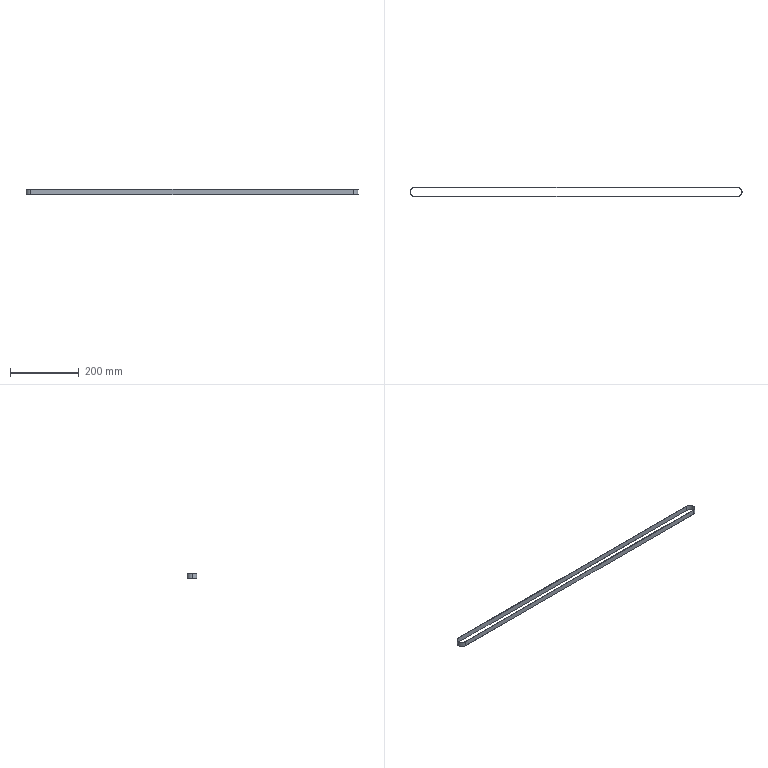Part | SolidWorks | features Extrusion 1 | 1 solid | 12 faces | box 965.34 x 28.34 x 15 mm | volume 34680 mm3 | cylinder 6 | plane 6 | commonest cylinder face diameters 25.98 x3 28.34 x3
STEP:
#1=CARTESIAN_POINT('',(0.,12.99,7.5));
#2=VERTEX_POINT('',#1);
#3=CARTESIAN_POINT('',(-12.99,0.,7.5));
#4=VERTEX_POINT('',#3);
#5=CARTESIAN_POINT('',(0.,0.,7.5));
#6=DIRECTION('',(0.,0.,1.));
#7=DIRECTION('',(1.,0.,0.));
#8=AXIS2_PLACEMENT_3D('',#5,#6,#7);
#9=CIRCLE('',#8,12.99);
#10=EDGE_CURVE('',#2,#4,#9,.T.);
#11=ORIENTED_EDGE('',*,*,#10,.T.);
#12=CARTESIAN_POINT('',(-12.99,0.,-7.5));
#13=VERTEX_POINT('',#12);
#14=CARTESIAN_POINT('',(-12.99,0.,7.5));
#15=DIRECTION('',(0.,0.,-1.));
#16=VECTOR('',#15,1000.);
#17=LINE('',#14,#16);
#18=EDGE_CURVE('',#4,#13,#17,.T.);
#19=ORIENTED_EDGE('',*,*,#18,.T.);
#20=CARTESIAN_POINT('',(0.,12.99,-7.5));
#21=VERTEX_POINT('',#20);
#22=CARTESIAN_POINT('',(0.,0.,-7.5));
#23=DIRECTION('',(0.,0.,1.));
#24=DIRECTION('',(1.,0.,0.));
#25=AXIS2_PLACEMENT_3D('',#22,#23,#24);
#26=CIRCLE('',#25,12.99);
#27=EDGE_CURVE('',#21,#13,#26,.T.);
#28=ORIENTED_EDGE('',*,*,#27,.F.);
#29=CARTESIAN_POINT('',(0.,12.99,7.5));
#30=DIRECTION('',(0.,0.,-1.));
#31=VECTOR('',#30,1000.);
#32=LINE('',#29,#31);
#33=EDGE_CURVE('',#2,#21,#32,.T.);
#34=ORIENTED_EDGE('',*,*,#33,.F.);
#35=EDGE_LOOP('',(#11,#19,#28,#34));
#36=FACE_OUTER_BOUND('',#35,.T.);
#37=CARTESIAN_POINT('',(0.,0.,7.5));
#38=DIRECTION('',(0.,0.,-1.));
#39=DIRECTION('',(-1.,0.,0.));
#40=AXIS2_PLACEMENT_3D('',#37,#38,#39);
#41=CYLINDRICAL_SURFACE('',#40,12.99);
#42=ADVANCED_FACE('',(#36),#41,.F.);
#43=CARTESIAN_POINT('',(-14.17,0.,7.5));
#44=VERTEX_POINT('',#43);
#45=CARTESIAN_POINT('',(0.,-14.17,7.5));
#46=VERTEX_POINT('',#45);
#47=CARTESIAN_POINT('',(0.,0.,7.5));
#48=DIRECTION('',(0.,0.,1.));
#49=DIRECTION('',(1.,0.,0.));
#50=AXIS2_PLACEMENT_3D('',#47,#48,#49);
#51=CIRCLE('',#50,14.17);
#52=EDGE_CURVE('',#44,#46,#51,.T.);
#53=ORIENTED_EDGE('',*,*,#52,.F.);
#54=CARTESIAN_POINT('',(-14.17,0.,-7.5));
#55=VERTEX_POINT('',#54);
#56=CARTESIAN_POINT('',(-14.17,0.,7.5));
#57=DIRECTION('',(0.,0.,-1.));
#58=VECTOR('',#57,1000.);
#59=LINE('',#56,#58);
#60=EDGE_CURVE('',#44,#55,#59,.T.);
#61=ORIENTED_EDGE('',*,*,#60,.T.);
#62=CARTESIAN_POINT('',(0.,-14.17,-7.5));
#63=VERTEX_POINT('',#62);
#64=CARTESIAN_POINT('',(0.,0.,-7.5));
#65=DIRECTION('',(0.,0.,1.));
#66=DIRECTION('',(1.,0.,0.));
#67=AXIS2_PLACEMENT_3D('',#64,#65,#66);
#68=CIRCLE('',#67,14.17);
#69=EDGE_CURVE('',#55,#63,#68,.T.);
#70=ORIENTED_EDGE('',*,*,#69,.T.);
#71=CARTESIAN_POINT('',(0.,-14.17,7.5));
#72=DIRECTION('',(0.,0.,-1.));
#73=VECTOR('',#72,1000.);
#74=LINE('',#71,#73);
#75=EDGE_CURVE('',#46,#63,#74,.T.);
#76=ORIENTED_EDGE('',*,*,#75,.F.);
#77=EDGE_LOOP('',(#53,#61,#70,#76));
#78=FACE_OUTER_BOUND('',#77,.T.);
#79=CARTESIAN_POINT('',(0.,0.,7.5));
#80=DIRECTION('',(0.,0.,-1.));
#81=DIRECTION('',(-1.,0.,0.));
#82=AXIS2_PLACEMENT_3D('',#79,#80,#81);
#83=CYLINDRICAL_SURFACE('',#82,14.17);
#84=ADVANCED_FACE('',(#78),#83,.T.);
#85=CARTESIAN_POINT('',(0.,14.17,7.5));
#86=VERTEX_POINT('',#85);
#87=CARTESIAN_POINT('',(0.,0.,7.5));
#88=DIRECTION('',(0.,0.,1.));
#89=DIRECTION('',(1.,0.,0.));
#90=AXIS2_PLACEMENT_3D('',#87,#88,#89);
#91=CIRCLE('',#90,14.17);
#92=EDGE_CURVE('',#86,#44,#91,.T.);
#93=ORIENTED_EDGE('',*,*,#92,.T.);
#94=ORIENTED_EDGE('',*,*,#52,.T.);
#95=CARTESIAN_POINT('',(937.,-14.17,7.5));
#96=VERTEX_POINT('',#95);
#97=CARTESIAN_POINT('',(937.,-14.17,7.5));
#98=DIRECTION('',(1.,0.,0.));
#99=VECTOR('',#98,1000.);
#100=LINE('',#97,#99);
#101=EDGE_CURVE('',#46,#96,#100,.T.);
#102=ORIENTED_EDGE('',*,*,#101,.T.);
#103=CARTESIAN_POINT('',(937.,14.17,7.5));
#104=VERTEX_POINT('',#103);
#105=CARTESIAN_POINT('',(937.,0.,7.5));
#106=DIRECTION('',(0.,0.,1.));
#107=DIRECTION('',(1.,0.,0.));
#108=AXIS2_PLACEMENT_3D('',#105,#106,#107);
#109=CIRCLE('',#108,14.17);
#110=EDGE_CURVE('',#96,#104,#109,.T.);
#111=ORIENTED_EDGE('',*,*,#110,.T.);
#112=CARTESIAN_POINT('',(0.,14.17,7.5));
#113=DIRECTION('',(-1.,0.,0.));
#114=VECTOR('',#113,1000.);
#115=LINE('',#112,#114);
#116=EDGE_CURVE('',#104,#86,#115,.T.);
#117=ORIENTED_EDGE('',*,*,#116,.T.);
#118=EDGE_LOOP('',(#93,#94,#102,#111,#117));
#119=FACE_OUTER_BOUND('',#118,.T.);
#120=CARTESIAN_POINT('',(0.,-12.99,7.5));
#121=VERTEX_POINT('',#120);
#122=CARTESIAN_POINT('',(937.,-12.99,7.5));
#123=VERTEX_POINT('',#122);
#124=CARTESIAN_POINT('',(937.,-12.99,7.5));
#125=DIRECTION('',(1.,0.,0.));
#126=VECTOR('',#125,1000.);
#127=LINE('',#124,#126);
#128=EDGE_CURVE('',#121,#123,#127,.T.);
#129=ORIENTED_EDGE('',*,*,#128,.F.);
#130=CARTESIAN_POINT('',(0.,0.,7.5));
#131=DIRECTION('',(0.,0.,1.));
#132=DIRECTION('',(1.,0.,0.));
#133=AXIS2_PLACEMENT_3D('',#130,#131,#132);
#134=CIRCLE('',#133,12.99);
#135=EDGE_CURVE('',#4,#121,#134,.T.);
#136=ORIENTED_EDGE('',*,*,#135,.F.);
#137=ORIENTED_EDGE('',*,*,#10,.F.);
#138=CARTESIAN_POINT('',(937.,12.99,7.5));
#139=VERTEX_POINT('',#138);
#140=CARTESIAN_POINT('',(0.,12.99,7.5));
#141=DIRECTION('',(-1.,0.,0.));
#142=VECTOR('',#141,1000.);
#143=LINE('',#140,#142);
#144=EDGE_CURVE('',#139,#2,#143,.T.);
#145=ORIENTED_EDGE('',*,*,#144,.F.);
#146=CARTESIAN_POINT('',(937.,0.,7.5));
#147=DIRECTION('',(0.,0.,1.));
#148=DIRECTION('',(1.,0.,0.));
#149=AXIS2_PLACEMENT_3D('',#146,#147,#148);
#150=CIRCLE('',#149,12.99);
#151=EDGE_CURVE('',#123,#139,#150,.T.);
#152=ORIENTED_EDGE('',*,*,#151,.F.);
#153=EDGE_LOOP('',(#129,#136,#137,#145,#152));
#154=FACE_BOUND('',#153,.T.);
#155=CARTESIAN_POINT('',(0.,0.,7.5));
#156=DIRECTION('',(0.,0.,1.));
#157=DIRECTION('',(1.,0.,0.));
#158=AXIS2_PLACEMENT_3D('',#155,#156,#157);
#159=PLANE('',#158);
#160=ADVANCED_FACE('',(#119,#154),#159,.T.);
#161=CARTESIAN_POINT('',(0.,14.17,-7.5));
#162=VERTEX_POINT('',#161);
#163=CARTESIAN_POINT('',(0.,0.,-7.5));
#164=DIRECTION('',(0.,0.,1.));
#165=DIRECTION('',(1.,0.,0.));
#166=AXIS2_PLACEMENT_3D('',#163,#164,#165);
#167=CIRCLE('',#166,14.17);
#168=EDGE_CURVE('',#162,#55,#167,.T.);
#169=ORIENTED_EDGE('',*,*,#168,.F.);
#170=CARTESIAN_POINT('',(937.,14.17,-7.5));
#171=VERTEX_POINT('',#170);
#172=CARTESIAN_POINT('',(0.,14.17,-7.5));
#173=DIRECTION('',(-1.,0.,0.));
#174=VECTOR('',#173,1000.);
#175=LINE('',#172,#174);
#176=EDGE_CURVE('',#171,#162,#175,.T.);
#177=ORIENTED_EDGE('',*,*,#176,.F.);
#178=CARTESIAN_POINT('',(937.,-14.17,-7.5));
#179=VERTEX_POINT('',#178);
#180=CARTESIAN_POINT('',(937.,0.,-7.5));
#181=DIRECTION('',(0.,0.,1.));
#182=DIRECTION('',(1.,0.,0.));
#183=AXIS2_PLACEMENT_3D('',#180,#181,#182);
#184=CIRCLE('',#183,14.17);
#185=EDGE_CURVE('',#179,#171,#184,.T.);
#186=ORIENTED_EDGE('',*,*,#185,.F.);
#187=CARTESIAN_POINT('',(937.,-14.17,-7.5));
#188=DIRECTION('',(1.,0.,0.));
#189=VECTOR('',#188,1000.);
#190=LINE('',#187,#189);
#191=EDGE_CURVE('',#63,#179,#190,.T.);
#192=ORIENTED_EDGE('',*,*,#191,.F.);
#193=ORIENTED_EDGE('',*,*,#69,.F.);
#194=EDGE_LOOP('',(#169,#177,#186,#192,#193));
#195=FACE_OUTER_BOUND('',#194,.T.);
#196=ORIENTED_EDGE('',*,*,#27,.T.);
#197=CARTESIAN_POINT('',(0.,-12.99,-7.5));
#198=VERTEX_POINT('',#197);
#199=CARTESIAN_POINT('',(0.,0.,-7.5));
#200=DIRECTION('',(0.,0.,1.));
#201=DIRECTION('',(1.,0.,0.));
#202=AXIS2_PLACEMENT_3D('',#199,#200,#201);
#203=CIRCLE('',#202,12.99);
#204=EDGE_CURVE('',#13,#198,#203,.T.);
#205=ORIENTED_EDGE('',*,*,#204,.T.);
#206=CARTESIAN_POINT('',(937.,-12.99,-7.5));
#207=VERTEX_POINT('',#206);
#208=CARTESIAN_POINT('',(937.,-12.99,-7.5));
#209=DIRECTION('',(1.,0.,0.));
#210=VECTOR('',#209,1000.);
#211=LINE('',#208,#210);
#212=EDGE_CURVE('',#198,#207,#211,.T.);
#213=ORIENTED_EDGE('',*,*,#212,.T.);
#214=CARTESIAN_POINT('',(937.,12.99,-7.5));
#215=VERTEX_POINT('',#214);
#216=CARTESIAN_POINT('',(937.,0.,-7.5));
#217=DIRECTION('',(0.,0.,1.));
#218=DIRECTION('',(1.,0.,0.));
#219=AXIS2_PLACEMENT_3D('',#216,#217,#218);
#220=CIRCLE('',#219,12.99);
#221=EDGE_CURVE('',#207,#215,#220,.T.);
#222=ORIENTED_EDGE('',*,*,#221,.T.);
#223=CARTESIAN_POINT('',(0.,12.99,-7.5));
#224=DIRECTION('',(-1.,0.,0.));
#225=VECTOR('',#224,1000.);
#226=LINE('',#223,#225);
#227=EDGE_CURVE('',#215,#21,#226,.T.);
#228=ORIENTED_EDGE('',*,*,#227,.T.);
#229=EDGE_LOOP('',(#196,#205,#213,#222,#228));
#230=FACE_BOUND('',#229,.T.);
#231=CARTESIAN_POINT('',(0.,0.,-7.5));
#232=DIRECTION('',(0.,0.,1.));
#233=DIRECTION('',(1.,0.,0.));
#234=AXIS2_PLACEMENT_3D('',#231,#232,#233);
#235=PLANE('',#234);
#236=ADVANCED_FACE('',(#195,#230),#235,.F.);
#237=ORIENTED_EDGE('',*,*,#60,.F.);
#238=ORIENTED_EDGE('',*,*,#92,.F.);
#239=CARTESIAN_POINT('',(0.,14.17,7.5));
#240=DIRECTION('',(0.,0.,-1.));
#241=VECTOR('',#240,1000.);
#242=LINE('',#239,#241);
#243=EDGE_CURVE('',#86,#162,#242,.T.);
#244=ORIENTED_EDGE('',*,*,#243,.T.);
#245=ORIENTED_EDGE('',*,*,#168,.T.);
#246=EDGE_LOOP('',(#237,#238,#244,#245));
#247=FACE_OUTER_BOUND('',#246,.T.);
#248=CARTESIAN_POINT('',(0.,0.,7.5));
#249=DIRECTION('',(0.,0.,-1.));
#250=DIRECTION('',(-1.,0.,0.));
#251=AXIS2_PLACEMENT_3D('',#248,#249,#250);
#252=CYLINDRICAL_SURFACE('',#251,14.17);
#253=ADVANCED_FACE('',(#247),#252,.T.);
#254=ORIENTED_EDGE('',*,*,#191,.T.);
#255=CARTESIAN_POINT('',(937.,-14.17,7.5));
#256=DIRECTION('',(0.,0.,-1.));
#257=VECTOR('',#256,1000.);
#258=LINE('',#255,#257);
#259=EDGE_CURVE('',#96,#179,#258,.T.);
#260=ORIENTED_EDGE('',*,*,#259,.F.);
#261=ORIENTED_EDGE('',*,*,#101,.F.);
#262=ORIENTED_EDGE('',*,*,#75,.T.);
#263=EDGE_LOOP('',(#254,#260,#261,#262));
#264=FACE_OUTER_BOUND('',#263,.T.);
#265=CARTESIAN_POINT('',(937.,-14.17,7.5));
#266=DIRECTION('',(0.,1.,0.));
#267=DIRECTION('',(0.,0.,1.));
#268=AXIS2_PLACEMENT_3D('',#265,#266,#267);
#269=PLANE('',#268);
#270=ADVANCED_FACE('',(#264),#269,.F.);
#271=ORIENTED_EDGE('',*,*,#185,.T.);
#272=CARTESIAN_POINT('',(937.,14.17,7.5));
#273=DIRECTION('',(0.,0.,-1.));
#274=VECTOR('',#273,1000.);
#275=LINE('',#272,#274);
#276=EDGE_CURVE('',#104,#171,#275,.T.);
#277=ORIENTED_EDGE('',*,*,#276,.F.);
#278=ORIENTED_EDGE('',*,*,#110,.F.);
#279=ORIENTED_EDGE('',*,*,#259,.T.);
#280=EDGE_LOOP('',(#271,#277,#278,#279));
#281=FACE_OUTER_BOUND('',#280,.T.);
#282=CARTESIAN_POINT('',(937.,0.,7.5));
#283=DIRECTION('',(0.,0.,-1.));
#284=DIRECTION('',(-1.,0.,0.));
#285=AXIS2_PLACEMENT_3D('',#282,#283,#284);
#286=CYLINDRICAL_SURFACE('',#285,14.17);
#287=ADVANCED_FACE('',(#281),#286,.T.);
#288=ORIENTED_EDGE('',*,*,#176,.T.);
#289=ORIENTED_EDGE('',*,*,#243,.F.);
#290=ORIENTED_EDGE('',*,*,#116,.F.);
#291=ORIENTED_EDGE('',*,*,#276,.T.);
#292=EDGE_LOOP('',(#288,#289,#290,#291));
#293=FACE_OUTER_BOUND('',#292,.T.);
#294=CARTESIAN_POINT('',(0.,14.17,7.5));
#295=DIRECTION('',(0.,-1.,0.));
#296=DIRECTION('',(0.,0.,-1.));
#297=AXIS2_PLACEMENT_3D('',#294,#295,#296);
#298=PLANE('',#297);
#299=ADVANCED_FACE('',(#293),#298,.F.);
#300=ORIENTED_EDGE('',*,*,#18,.F.);
#301=ORIENTED_EDGE('',*,*,#135,.T.);
#302=CARTESIAN_POINT('',(0.,-12.99,7.5));
#303=DIRECTION('',(0.,0.,-1.));
#304=VECTOR('',#303,1000.);
#305=LINE('',#302,#304);
#306=EDGE_CURVE('',#121,#198,#305,.T.);
#307=ORIENTED_EDGE('',*,*,#306,.T.);
#308=ORIENTED_EDGE('',*,*,#204,.F.);
#309=EDGE_LOOP('',(#300,#301,#307,#308));
#310=FACE_OUTER_BOUND('',#309,.T.);
#311=CARTESIAN_POINT('',(0.,0.,7.5));
#312=DIRECTION('',(0.,0.,-1.));
#313=DIRECTION('',(-1.,0.,0.));
#314=AXIS2_PLACEMENT_3D('',#311,#312,#313);
#315=CYLINDRICAL_SURFACE('',#314,12.99);
#316=ADVANCED_FACE('',(#310),#315,.F.);
#317=ORIENTED_EDGE('',*,*,#212,.F.);
#318=ORIENTED_EDGE('',*,*,#306,.F.);
#319=ORIENTED_EDGE('',*,*,#128,.T.);
#320=CARTESIAN_POINT('',(937.,-12.99,7.5));
#321=DIRECTION('',(0.,0.,-1.));
#322=VECTOR('',#321,1000.);
#323=LINE('',#320,#322);
#324=EDGE_CURVE('',#123,#207,#323,.T.);
#325=ORIENTED_EDGE('',*,*,#324,.T.);
#326=EDGE_LOOP('',(#317,#318,#319,#325));
#327=FACE_OUTER_BOUND('',#326,.T.);
#328=CARTESIAN_POINT('',(937.,-12.99,7.5));
#329=DIRECTION('',(0.,1.,0.));
#330=DIRECTION('',(0.,0.,1.));
#331=AXIS2_PLACEMENT_3D('',#328,#329,#330);
#332=PLANE('',#331);
#333=ADVANCED_FACE('',(#327),#332,.T.);
#334=ORIENTED_EDGE('',*,*,#221,.F.);
#335=ORIENTED_EDGE('',*,*,#324,.F.);
#336=ORIENTED_EDGE('',*,*,#151,.T.);
#337=CARTESIAN_POINT('',(937.,12.99,7.5));
#338=DIRECTION('',(0.,0.,-1.));
#339=VECTOR('',#338,1000.);
#340=LINE('',#337,#339);
#341=EDGE_CURVE('',#139,#215,#340,.T.);
#342=ORIENTED_EDGE('',*,*,#341,.T.);
#343=EDGE_LOOP('',(#334,#335,#336,#342));
#344=FACE_OUTER_BOUND('',#343,.T.);
#345=CARTESIAN_POINT('',(937.,0.,7.5));
#346=DIRECTION('',(0.,0.,-1.));
#347=DIRECTION('',(-1.,0.,0.));
#348=AXIS2_PLACEMENT_3D('',#345,#346,#347);
#349=CYLINDRICAL_SURFACE('',#348,12.99);
#350=ADVANCED_FACE('',(#344),#349,.F.);
#351=ORIENTED_EDGE('',*,*,#227,.F.);
#352=ORIENTED_EDGE('',*,*,#341,.F.);
#353=ORIENTED_EDGE('',*,*,#144,.T.);
#354=ORIENTED_EDGE('',*,*,#33,.T.);
#355=EDGE_LOOP('',(#351,#352,#353,#354));
#356=FACE_OUTER_BOUND('',#355,.T.);
#357=CARTESIAN_POINT('',(0.,12.99,7.5));
#358=DIRECTION('',(0.,-1.,0.));
#359=DIRECTION('',(0.,0.,-1.));
#360=AXIS2_PLACEMENT_3D('',#357,#358,#359);
#361=PLANE('',#360);
#362=ADVANCED_FACE('',(#356),#361,.T.);
#363=CLOSED_SHELL('',(#42,#84,#160,#236,#253,#270,#287,#299,#316,#333,#350,#362));
#364=MANIFOLD_SOLID_BREP('',#363);
#365=CARTESIAN_POINT('',(0.,0.,0.));
#366=DIRECTION('',(0.,0.,1.));
#367=DIRECTION('',(1.,0.,0.));
#368=AXIS2_PLACEMENT_3D('',#365,#366,#367);
#369=(LENGTH_UNIT()NAMED_UNIT(*)SI_UNIT(.MILLI.,.METRE.));
#370=UNCERTAINTY_MEASURE_WITH_UNIT(LENGTH_MEASURE(0.00001),#369,'','');
#371=(NAMED_UNIT(*)PLANE_ANGLE_UNIT()SI_UNIT($,.RADIAN.));
#372=(NAMED_UNIT(*)SI_UNIT($,.STERADIAN.)SOLID_ANGLE_UNIT());
#373=(GEOMETRIC_REPRESENTATION_CONTEXT(3)GLOBAL_UNCERTAINTY_ASSIGNED_CONTEXT((#370))GLOBAL_UNIT_ASSIGNED_CONTEXT((#369,#371,#372))REPRESENTATION_CONTEXT('',''));
#374=ADVANCED_BREP_SHAPE_REPRESENTATION('',(#364,#368),#373);